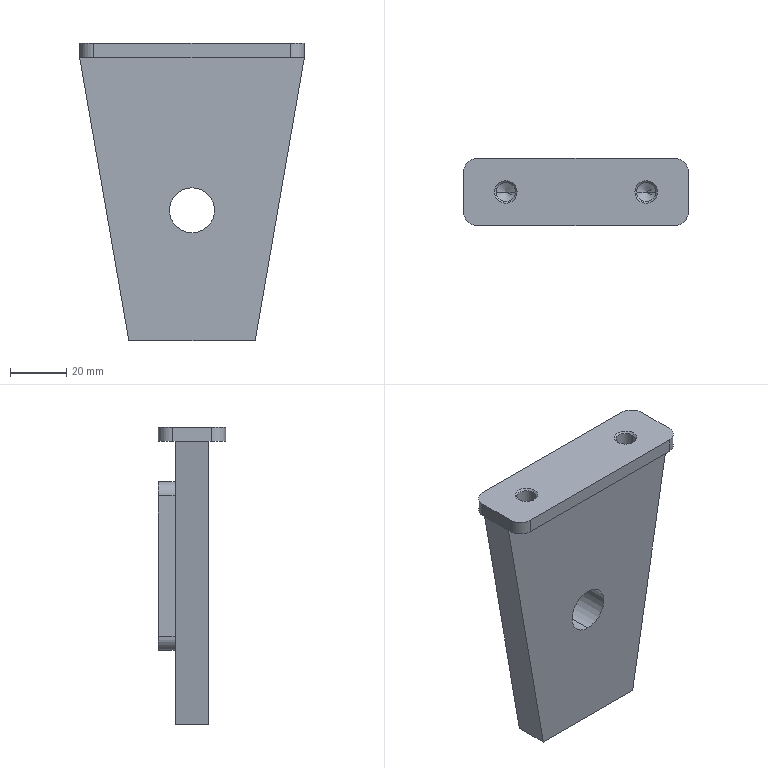Part | SolidWorks | features ICE 3, 3DProfileFeature 2, HoleWzd 2, Extrusion 1 | 1 solid | 51 faces | box 80 x 24 x 106 mm | volume 92527 mm3 | cylinder 18 | plane 17 | cone 16 | commonest cylinder face diameters 10 x8 5 x4 6.8 x4 16 x2
STEP:
#1=CARTESIAN_POINT('',(16.5,0.,-100.475));
#2=VERTEX_POINT('',#1);
#3=CARTESIAN_POINT('',(11.5,0.,-100.475));
#4=VERTEX_POINT('',#3);
#5=CARTESIAN_POINT('',(14.,0.,-100.475));
#6=DIRECTION('',(0.,0.,-1.));
#7=DIRECTION('',(-1.,0.,0.));
#8=AXIS2_PLACEMENT_3D('',#5,#6,#7);
#9=CIRCLE('',#8,2.5);
#10=EDGE_CURVE('',#2,#4,#9,.T.);
#11=ORIENTED_EDGE('',*,*,#10,.F.);
#12=CARTESIAN_POINT('',(17.025,0.,-101.));
#13=VERTEX_POINT('',#12);
#14=CARTESIAN_POINT('',(17.025,0.,-101.));
#15=DIRECTION('',(0.7071,0.,-0.7071));
#16=VECTOR('',#15,1000.);
#17=LINE('',#14,#16);
#18=EDGE_CURVE('',#2,#13,#17,.T.);
#19=ORIENTED_EDGE('',*,*,#18,.T.);
#20=CARTESIAN_POINT('',(10.975,0.,-101.));
#21=VERTEX_POINT('',#20);
#22=CARTESIAN_POINT('',(14.,0.,-101.));
#23=DIRECTION('',(0.,0.,-1.));
#24=DIRECTION('',(-1.,0.,0.));
#25=AXIS2_PLACEMENT_3D('',#22,#23,#24);
#26=CIRCLE('',#25,3.025);
#27=EDGE_CURVE('',#13,#21,#26,.T.);
#28=ORIENTED_EDGE('',*,*,#27,.T.);
#29=CARTESIAN_POINT('',(10.975,0.,-101.));
#30=DIRECTION('',(-0.7071,0.,-0.7071));
#31=VECTOR('',#30,1000.);
#32=LINE('',#29,#31);
#33=EDGE_CURVE('',#4,#21,#32,.T.);
#34=ORIENTED_EDGE('',*,*,#33,.F.);
#35=EDGE_LOOP('',(#11,#19,#28,#34));
#36=FACE_OUTER_BOUND('',#35,.T.);
#37=CARTESIAN_POINT('',(14.,0.,-101.));
#38=DIRECTION('',(0.,0.,-1.));
#39=DIRECTION('',(-1.,0.,0.));
#40=AXIS2_PLACEMENT_3D('',#37,#38,#39);
#41=CONICAL_SURFACE('',#40,3.025,0.7854);
#42=ADVANCED_FACE('',(#36),#41,.F.);
#43=CARTESIAN_POINT('',(16.5,0.,-91.));
#44=VERTEX_POINT('',#43);
#45=CARTESIAN_POINT('',(11.5,0.,-91.));
#46=VERTEX_POINT('',#45);
#47=CARTESIAN_POINT('',(14.,0.,-91.));
#48=DIRECTION('',(0.,0.,-1.));
#49=DIRECTION('',(-1.,0.,0.));
#50=AXIS2_PLACEMENT_3D('',#47,#48,#49);
#51=CIRCLE('',#50,2.5);
#52=EDGE_CURVE('',#44,#46,#51,.T.);
#53=ORIENTED_EDGE('',*,*,#52,.F.);
#54=CARTESIAN_POINT('',(16.5,0.,-101.));
#55=DIRECTION('',(0.,0.,-1.));
#56=VECTOR('',#55,1000.);
#57=LINE('',#54,#56);
#58=EDGE_CURVE('',#44,#2,#57,.T.);
#59=ORIENTED_EDGE('',*,*,#58,.T.);
#60=ORIENTED_EDGE('',*,*,#10,.T.);
#61=CARTESIAN_POINT('',(11.5,0.,-101.));
#62=DIRECTION('',(0.,0.,-1.));
#63=VECTOR('',#62,1000.);
#64=LINE('',#61,#63);
#65=EDGE_CURVE('',#46,#4,#64,.T.);
#66=ORIENTED_EDGE('',*,*,#65,.F.);
#67=EDGE_LOOP('',(#53,#59,#60,#66));
#68=FACE_OUTER_BOUND('',#67,.T.);
#69=CARTESIAN_POINT('',(14.,0.,-101.));
#70=DIRECTION('',(0.,0.,-1.));
#71=DIRECTION('',(-1.,0.,0.));
#72=AXIS2_PLACEMENT_3D('',#69,#70,#71);
#73=CYLINDRICAL_SURFACE('',#72,2.5);
#74=ADVANCED_FACE('',(#68),#73,.F.);
#75=CARTESIAN_POINT('',(14.,0.,-89.498));
#76=VERTEX_POINT('',#75);
#77=CARTESIAN_POINT('',(11.5,0.,-91.));
#78=DIRECTION('',(-0.8572,0.,-0.515));
#79=VECTOR('',#78,1000.);
#80=LINE('',#77,#79);
#81=EDGE_CURVE('',#76,#46,#80,.T.);
#82=ORIENTED_EDGE('',*,*,#81,.F.);
#83=CARTESIAN_POINT('',(16.5,0.,-91.));
#84=DIRECTION('',(0.8572,0.,-0.515));
#85=VECTOR('',#84,1000.);
#86=LINE('',#83,#85);
#87=EDGE_CURVE('',#76,#44,#86,.T.);
#88=ORIENTED_EDGE('',*,*,#87,.T.);
#89=ORIENTED_EDGE('',*,*,#52,.T.);
#90=EDGE_LOOP('',(#82,#88,#89));
#91=FACE_OUTER_BOUND('',#90,.T.);
#92=CARTESIAN_POINT('',(14.,0.,-91.));
#93=DIRECTION('',(0.,0.,-1.));
#94=DIRECTION('',(-1.,0.,0.));
#95=AXIS2_PLACEMENT_3D('',#92,#93,#94);
#96=CONICAL_SURFACE('',#95,2.5,1.03);
#97=ADVANCED_FACE('',(#91),#96,.F.);
#98=CARTESIAN_POINT('',(-11.5,0.,-100.475));
#99=VERTEX_POINT('',#98);
#100=CARTESIAN_POINT('',(-16.5,0.,-100.475));
#101=VERTEX_POINT('',#100);
#102=CARTESIAN_POINT('',(-14.,0.,-100.475));
#103=DIRECTION('',(0.,0.,-1.));
#104=DIRECTION('',(-1.,0.,0.));
#105=AXIS2_PLACEMENT_3D('',#102,#103,#104);
#106=CIRCLE('',#105,2.5);
#107=EDGE_CURVE('',#99,#101,#106,.T.);
#108=ORIENTED_EDGE('',*,*,#107,.F.);
#109=CARTESIAN_POINT('',(-10.975,0.,-101.));
#110=VERTEX_POINT('',#109);
#111=CARTESIAN_POINT('',(-10.975,0.,-101.));
#112=DIRECTION('',(0.7071,0.,-0.7071));
#113=VECTOR('',#112,1000.);
#114=LINE('',#111,#113);
#115=EDGE_CURVE('',#99,#110,#114,.T.);
#116=ORIENTED_EDGE('',*,*,#115,.T.);
#117=CARTESIAN_POINT('',(-17.025,0.,-101.));
#118=VERTEX_POINT('',#117);
#119=CARTESIAN_POINT('',(-14.,0.,-101.));
#120=DIRECTION('',(0.,0.,-1.));
#121=DIRECTION('',(-1.,0.,0.));
#122=AXIS2_PLACEMENT_3D('',#119,#120,#121);
#123=CIRCLE('',#122,3.025);
#124=EDGE_CURVE('',#110,#118,#123,.T.);
#125=ORIENTED_EDGE('',*,*,#124,.T.);
#126=CARTESIAN_POINT('',(-17.025,0.,-101.));
#127=DIRECTION('',(-0.7071,0.,-0.7071));
#128=VECTOR('',#127,1000.);
#129=LINE('',#126,#128);
#130=EDGE_CURVE('',#101,#118,#129,.T.);
#131=ORIENTED_EDGE('',*,*,#130,.F.);
#132=EDGE_LOOP('',(#108,#116,#125,#131));
#133=FACE_OUTER_BOUND('',#132,.T.);
#134=CARTESIAN_POINT('',(-14.,0.,-101.));
#135=DIRECTION('',(0.,0.,-1.));
#136=DIRECTION('',(-1.,0.,0.));
#137=AXIS2_PLACEMENT_3D('',#134,#135,#136);
#138=CONICAL_SURFACE('',#137,3.025,0.7854);
#139=ADVANCED_FACE('',(#133),#138,.F.);
#140=CARTESIAN_POINT('',(-11.5,0.,-91.));
#141=VERTEX_POINT('',#140);
#142=CARTESIAN_POINT('',(-16.5,0.,-91.));
#143=VERTEX_POINT('',#142);
#144=CARTESIAN_POINT('',(-14.,0.,-91.));
#145=DIRECTION('',(0.,0.,-1.));
#146=DIRECTION('',(-1.,0.,0.));
#147=AXIS2_PLACEMENT_3D('',#144,#145,#146);
#148=CIRCLE('',#147,2.5);
#149=EDGE_CURVE('',#141,#143,#148,.T.);
#150=ORIENTED_EDGE('',*,*,#149,.F.);
#151=CARTESIAN_POINT('',(-11.5,0.,-101.));
#152=DIRECTION('',(0.,0.,-1.));
#153=VECTOR('',#152,1000.);
#154=LINE('',#151,#153);
#155=EDGE_CURVE('',#141,#99,#154,.T.);
#156=ORIENTED_EDGE('',*,*,#155,.T.);
#157=ORIENTED_EDGE('',*,*,#107,.T.);
#158=CARTESIAN_POINT('',(-16.5,0.,-101.));
#159=DIRECTION('',(0.,0.,-1.));
#160=VECTOR('',#159,1000.);
#161=LINE('',#158,#160);
#162=EDGE_CURVE('',#143,#101,#161,.T.);
#163=ORIENTED_EDGE('',*,*,#162,.F.);
#164=EDGE_LOOP('',(#150,#156,#157,#163));
#165=FACE_OUTER_BOUND('',#164,.T.);
#166=CARTESIAN_POINT('',(-14.,0.,-101.));
#167=DIRECTION('',(0.,0.,-1.));
#168=DIRECTION('',(-1.,0.,0.));
#169=AXIS2_PLACEMENT_3D('',#166,#167,#168);
#170=CYLINDRICAL_SURFACE('',#169,2.5);
#171=ADVANCED_FACE('',(#165),#170,.F.);
#172=CARTESIAN_POINT('',(-14.,0.,-89.498));
#173=VERTEX_POINT('',#172);
#174=CARTESIAN_POINT('',(-16.5,0.,-91.));
#175=DIRECTION('',(-0.8572,0.,-0.515));
#176=VECTOR('',#175,1000.);
#177=LINE('',#174,#176);
#178=EDGE_CURVE('',#173,#143,#177,.T.);
#179=ORIENTED_EDGE('',*,*,#178,.F.);
#180=CARTESIAN_POINT('',(-11.5,0.,-91.));
#181=DIRECTION('',(0.8572,0.,-0.515));
#182=VECTOR('',#181,1000.);
#183=LINE('',#180,#182);
#184=EDGE_CURVE('',#173,#141,#183,.T.);
#185=ORIENTED_EDGE('',*,*,#184,.T.);
#186=ORIENTED_EDGE('',*,*,#149,.T.);
#187=EDGE_LOOP('',(#179,#185,#186));
#188=FACE_OUTER_BOUND('',#187,.T.);
#189=CARTESIAN_POINT('',(-14.,0.,-91.));
#190=DIRECTION('',(0.,0.,-1.));
#191=DIRECTION('',(-1.,0.,0.));
#192=AXIS2_PLACEMENT_3D('',#189,#190,#191);
#193=CONICAL_SURFACE('',#192,2.5,1.03);
#194=ADVANCED_FACE('',(#188),#193,.F.);
#195=CARTESIAN_POINT('',(21.6,0.,4.375));
#196=VERTEX_POINT('',#195);
#197=CARTESIAN_POINT('',(28.4,0.,4.375));
#198=VERTEX_POINT('',#197);
#199=CARTESIAN_POINT('',(25.,0.,4.375));
#200=DIRECTION('',(0.,0.,1.));
#201=DIRECTION('',(1.,0.,0.));
#202=AXIS2_PLACEMENT_3D('',#199,#200,#201);
#203=CIRCLE('',#202,3.4);
#204=EDGE_CURVE('',#196,#198,#203,.T.);
#205=ORIENTED_EDGE('',*,*,#204,.F.);
#206=CARTESIAN_POINT('',(20.975,0.,5.));
#207=VERTEX_POINT('',#206);
#208=CARTESIAN_POINT('',(20.975,0.,5.));
#209=DIRECTION('',(-0.7071,0.,0.7071));
#210=VECTOR('',#209,1000.);
#211=LINE('',#208,#210);
#212=EDGE_CURVE('',#196,#207,#211,.T.);
#213=ORIENTED_EDGE('',*,*,#212,.T.);
#214=CARTESIAN_POINT('',(29.025,0.,5.));
#215=VERTEX_POINT('',#214);
#216=CARTESIAN_POINT('',(25.,0.,5.));
#217=DIRECTION('',(0.,0.,1.));
#218=DIRECTION('',(1.,0.,0.));
#219=AXIS2_PLACEMENT_3D('',#216,#217,#218);
#220=CIRCLE('',#219,4.025);
#221=EDGE_CURVE('',#207,#215,#220,.T.);
#222=ORIENTED_EDGE('',*,*,#221,.T.);
#223=CARTESIAN_POINT('',(29.025,0.,5.));
#224=DIRECTION('',(0.7071,0.,0.7071));
#225=VECTOR('',#224,1000.);
#226=LINE('',#223,#225);
#227=EDGE_CURVE('',#198,#215,#226,.T.);
#228=ORIENTED_EDGE('',*,*,#227,.F.);
#229=EDGE_LOOP('',(#205,#213,#222,#228));
#230=FACE_OUTER_BOUND('',#229,.T.);
#231=CARTESIAN_POINT('',(25.,0.,5.));
#232=DIRECTION('',(0.,0.,1.));
#233=DIRECTION('',(1.,0.,0.));
#234=AXIS2_PLACEMENT_3D('',#231,#232,#233);
#235=CONICAL_SURFACE('',#234,4.025,0.7854);
#236=ADVANCED_FACE('',(#230),#235,.F.);
#237=CARTESIAN_POINT('',(21.6,0.,-15.));
#238=VERTEX_POINT('',#237);
#239=CARTESIAN_POINT('',(28.4,0.,-15.));
#240=VERTEX_POINT('',#239);
#241=CARTESIAN_POINT('',(25.,0.,-15.));
#242=DIRECTION('',(0.,0.,1.));
#243=DIRECTION('',(1.,0.,0.));
#244=AXIS2_PLACEMENT_3D('',#241,#242,#243);
#245=CIRCLE('',#244,3.4);
#246=EDGE_CURVE('',#238,#240,#245,.T.);
#247=ORIENTED_EDGE('',*,*,#246,.F.);
#248=CARTESIAN_POINT('',(21.6,0.,5.));
#249=DIRECTION('',(0.,0.,1.));
#250=VECTOR('',#249,1000.);
#251=LINE('',#248,#250);
#252=EDGE_CURVE('',#238,#196,#251,.T.);
#253=ORIENTED_EDGE('',*,*,#252,.T.);
#254=ORIENTED_EDGE('',*,*,#204,.T.);
#255=CARTESIAN_POINT('',(28.4,0.,5.));
#256=DIRECTION('',(0.,0.,1.));
#257=VECTOR('',#256,1000.);
#258=LINE('',#255,#257);
#259=EDGE_CURVE('',#240,#198,#258,.T.);
#260=ORIENTED_EDGE('',*,*,#259,.F.);
#261=EDGE_LOOP('',(#247,#253,#254,#260));
#262=FACE_OUTER_BOUND('',#261,.T.);
#263=CARTESIAN_POINT('',(25.,0.,5.));
#264=DIRECTION('',(0.,0.,1.));
#265=DIRECTION('',(1.,0.,0.));
#266=AXIS2_PLACEMENT_3D('',#263,#264,#265);
#267=CYLINDRICAL_SURFACE('',#266,3.4);
#268=ADVANCED_FACE('',(#262),#267,.F.);
#269=CARTESIAN_POINT('',(25.,0.,-17.043));
#270=VERTEX_POINT('',#269);
#271=CARTESIAN_POINT('',(28.4,0.,-15.));
#272=DIRECTION('',(0.8572,0.,0.515));
#273=VECTOR('',#272,1000.);
#274=LINE('',#271,#273);
#275=EDGE_CURVE('',#270,#240,#274,.T.);
#276=ORIENTED_EDGE('',*,*,#275,.F.);
#277=CARTESIAN_POINT('',(21.6,0.,-15.));
#278=DIRECTION('',(-0.8572,0.,0.515));
#279=VECTOR('',#278,1000.);
#280=LINE('',#277,#279);
#281=EDGE_CURVE('',#270,#238,#280,.T.);
#282=ORIENTED_EDGE('',*,*,#281,.T.);
#283=ORIENTED_EDGE('',*,*,#246,.T.);
#284=EDGE_LOOP('',(#276,#282,#283));
#285=FACE_OUTER_BOUND('',#284,.T.);
#286=CARTESIAN_POINT('',(25.,0.,-15.));
#287=DIRECTION('',(0.,0.,1.));
#288=DIRECTION('',(1.,0.,0.));
#289=AXIS2_PLACEMENT_3D('',#286,#287,#288);
#290=CONICAL_SURFACE('',#289,3.4,1.03);
#291=ADVANCED_FACE('',(#285),#290,.F.);
#292=CARTESIAN_POINT('',(-28.4,0.,4.375));
#293=VERTEX_POINT('',#292);
#294=CARTESIAN_POINT('',(-21.6,0.,4.375));
#295=VERTEX_POINT('',#294);
#296=CARTESIAN_POINT('',(-25.,0.,4.375));
#297=DIRECTION('',(0.,0.,1.));
#298=DIRECTION('',(1.,0.,0.));
#299=AXIS2_PLACEMENT_3D('',#296,#297,#298);
#300=CIRCLE('',#299,3.4);
#301=EDGE_CURVE('',#293,#295,#300,.T.);
#302=ORIENTED_EDGE('',*,*,#301,.F.);
#303=CARTESIAN_POINT('',(-29.025,0.,5.));
#304=VERTEX_POINT('',#303);
#305=CARTESIAN_POINT('',(-29.025,0.,5.));
#306=DIRECTION('',(-0.7071,0.,0.7071));
#307=VECTOR('',#306,1000.);
#308=LINE('',#305,#307);
#309=EDGE_CURVE('',#293,#304,#308,.T.);
#310=ORIENTED_EDGE('',*,*,#309,.T.);
#311=CARTESIAN_POINT('',(-20.975,0.,5.));
#312=VERTEX_POINT('',#311);
#313=CARTESIAN_POINT('',(-25.,0.,5.));
#314=DIRECTION('',(0.,0.,1.));
#315=DIRECTION('',(1.,0.,0.));
#316=AXIS2_PLACEMENT_3D('',#313,#314,#315);
#317=CIRCLE('',#316,4.025);
#318=EDGE_CURVE('',#304,#312,#317,.T.);
#319=ORIENTED_EDGE('',*,*,#318,.T.);
#320=CARTESIAN_POINT('',(-20.975,0.,5.));
#321=DIRECTION('',(0.7071,0.,0.7071));
#322=VECTOR('',#321,1000.);
#323=LINE('',#320,#322);
#324=EDGE_CURVE('',#295,#312,#323,.T.);
#325=ORIENTED_EDGE('',*,*,#324,.F.);
#326=EDGE_LOOP('',(#302,#310,#319,#325));
#327=FACE_OUTER_BOUND('',#326,.T.);
#328=CARTESIAN_POINT('',(-25.,0.,5.));
#329=DIRECTION('',(0.,0.,1.));
#330=DIRECTION('',(1.,0.,0.));
#331=AXIS2_PLACEMENT_3D('',#328,#329,#330);
#332=CONICAL_SURFACE('',#331,4.025,0.7854);
#333=ADVANCED_FACE('',(#327),#332,.F.);
#334=CARTESIAN_POINT('',(-28.4,0.,-15.));
#335=VERTEX_POINT('',#334);
#336=CARTESIAN_POINT('',(-21.6,0.,-15.));
#337=VERTEX_POINT('',#336);
#338=CARTESIAN_POINT('',(-25.,0.,-15.));
#339=DIRECTION('',(0.,0.,1.));
#340=DIRECTION('',(1.,0.,0.));
#341=AXIS2_PLACEMENT_3D('',#338,#339,#340);
#342=CIRCLE('',#341,3.4);
#343=EDGE_CURVE('',#335,#337,#342,.T.);
#344=ORIENTED_EDGE('',*,*,#343,.F.);
#345=CARTESIAN_POINT('',(-28.4,0.,5.));
#346=DIRECTION('',(0.,0.,1.));
#347=VECTOR('',#346,1000.);
#348=LINE('',#345,#347);
#349=EDGE_CURVE('',#335,#293,#348,.T.);
#350=ORIENTED_EDGE('',*,*,#349,.T.);
#351=ORIENTED_EDGE('',*,*,#301,.T.);
#352=CARTESIAN_POINT('',(-21.6,0.,5.));
#353=DIRECTION('',(0.,0.,1.));
#354=VECTOR('',#353,1000.);
#355=LINE('',#352,#354);
#356=EDGE_CURVE('',#337,#295,#355,.T.);
#357=ORIENTED_EDGE('',*,*,#356,.F.);
#358=EDGE_LOOP('',(#344,#350,#351,#357));
#359=FACE_OUTER_BOUND('',#358,.T.);
#360=CARTESIAN_POINT('',(-25.,0.,5.));
#361=DIRECTION('',(0.,0.,1.));
#362=DIRECTION('',(1.,0.,0.));
#363=AXIS2_PLACEMENT_3D('',#360,#361,#362);
#364=CYLINDRICAL_SURFACE('',#363,3.4);
#365=ADVANCED_FACE('',(#359),#364,.F.);
#366=CARTESIAN_POINT('',(-25.,0.,-17.043));
#367=VERTEX_POINT('',#366);
#368=CARTESIAN_POINT('',(-21.6,0.,-15.));
#369=DIRECTION('',(0.8572,0.,0.515));
#370=VECTOR('',#369,1000.);
#371=LINE('',#368,#370);
#372=EDGE_CURVE('',#367,#337,#371,.T.);
#373=ORIENTED_EDGE('',*,*,#372,.F.);
#374=CARTESIAN_POINT('',(-28.4,0.,-15.));
#375=DIRECTION('',(-0.8572,0.,0.515));
#376=VECTOR('',#375,1000.);
#377=LINE('',#374,#376);
#378=EDGE_CURVE('',#367,#335,#377,.T.);
#379=ORIENTED_EDGE('',*,*,#378,.T.);
#380=ORIENTED_EDGE('',*,*,#343,.T.);
#381=EDGE_LOOP('',(#373,#379,#380));
#382=FACE_OUTER_BOUND('',#381,.T.);
#383=CARTESIAN_POINT('',(-25.,0.,-15.));
#384=DIRECTION('',(0.,0.,1.));
#385=DIRECTION('',(1.,0.,0.));
#386=AXIS2_PLACEMENT_3D('',#383,#384,#385);
#387=CONICAL_SURFACE('',#386,3.4,1.03);
#388=ADVANCED_FACE('',(#382),#387,.F.);
#389=CARTESIAN_POINT('',(0.,-6.,-46.5));
#390=VERTEX_POINT('',#389);
#391=CARTESIAN_POINT('',(0.,-6.,-62.5));
#392=VERTEX_POINT('',#391);
#393=CARTESIAN_POINT('',(0.,-6.,-54.5));
#394=DIRECTION('',(0.,-1.,0.));
#395=DIRECTION('',(0.,0.,-1.));
#396=AXIS2_PLACEMENT_3D('',#393,#394,#395);
#397=CIRCLE('',#396,8.);
#398=EDGE_CURVE('',#390,#392,#397,.T.);
#399=ORIENTED_EDGE('',*,*,#398,.T.);
#400=CARTESIAN_POINT('',(0.,12.,-62.5));
#401=VERTEX_POINT('',#400);
#402=CARTESIAN_POINT('',(0.,-9.,-62.5));
#403=DIRECTION('',(0.,1.,0.));
#404=VECTOR('',#403,1000.);
#405=LINE('',#402,#404);
#406=EDGE_CURVE('',#392,#401,#405,.T.);
#407=ORIENTED_EDGE('',*,*,#406,.T.);
#408=CARTESIAN_POINT('',(0.,12.,-46.5));
#409=VERTEX_POINT('',#408);
#410=CARTESIAN_POINT('',(0.,12.,-54.5));
#411=DIRECTION('',(0.,1.,0.));
#412=DIRECTION('',(0.,0.,1.));
#413=AXIS2_PLACEMENT_3D('',#410,#411,#412);
#414=CIRCLE('',#413,8.);
#415=EDGE_CURVE('',#401,#409,#414,.T.);
#416=ORIENTED_EDGE('',*,*,#415,.T.);
#417=CARTESIAN_POINT('',(0.,-9.,-46.5));
#418=DIRECTION('',(0.,1.,0.));
#419=VECTOR('',#418,1000.);
#420=LINE('',#417,#419);
#421=EDGE_CURVE('',#390,#409,#420,.T.);
#422=ORIENTED_EDGE('',*,*,#421,.F.);
#423=EDGE_LOOP('',(#399,#407,#416,#422));
#424=FACE_OUTER_BOUND('',#423,.T.);
#425=CARTESIAN_POINT('',(0.,-9.,-54.5));
#426=DIRECTION('',(0.,1.,0.));
#427=DIRECTION('',(0.,0.,1.));
#428=AXIS2_PLACEMENT_3D('',#425,#426,#427);
#429=CYLINDRICAL_SURFACE('',#428,8.);
#430=ADVANCED_FACE('',(#424),#429,.F.);
#431=CARTESIAN_POINT('',(-40.,6.,0.));
#432=VERTEX_POINT('',#431);
#433=CARTESIAN_POINT('',(40.,6.,0.));
#434=VERTEX_POINT('',#433);
#435=CARTESIAN_POINT('',(40.,6.,0.));
#436=DIRECTION('',(1.,0.,0.));
#437=VECTOR('',#436,1000.);
#438=LINE('',#435,#437);
#439=EDGE_CURVE('',#432,#434,#438,.T.);
#440=ORIENTED_EDGE('',*,*,#439,.T.);
#441=CARTESIAN_POINT('',(22.5,6.,-101.));
#442=VERTEX_POINT('',#441);
#443=CARTESIAN_POINT('',(22.5,6.,-101.));
#444=DIRECTION('',(-0.1707,0.,-0.9853));
#445=VECTOR('',#444,1000.);
#446=LINE('',#443,#445);
#447=EDGE_CURVE('',#434,#442,#446,.T.);
#448=ORIENTED_EDGE('',*,*,#447,.T.);
#449=CARTESIAN_POINT('',(-22.5,6.,-101.));
#450=VERTEX_POINT('',#449);
#451=CARTESIAN_POINT('',(-22.5,6.,-101.));
#452=DIRECTION('',(-1.,0.,0.));
#453=VECTOR('',#452,1000.);
#454=LINE('',#451,#453);
#455=EDGE_CURVE('',#442,#450,#454,.T.);
#456=ORIENTED_EDGE('',*,*,#455,.T.);
#457=CARTESIAN_POINT('',(-40.,6.,0.));
#458=DIRECTION('',(-0.1707,0.,0.9853));
#459=VECTOR('',#458,1000.);
#460=LINE('',#457,#459);
#461=EDGE_CURVE('',#450,#432,#460,.T.);
#462=ORIENTED_EDGE('',*,*,#461,.T.);
#463=EDGE_LOOP('',(#440,#448,#456,#462));
#464=FACE_OUTER_BOUND('',#463,.T.);
#465=CARTESIAN_POINT('',(-18.,6.,-19.5));
#466=VERTEX_POINT('',#465);
#467=CARTESIAN_POINT('',(-13.,6.,-14.5));
#468=VERTEX_POINT('',#467);
#469=CARTESIAN_POINT('',(-13.,6.,-19.5));
#470=DIRECTION('',(0.,1.,0.));
#471=DIRECTION('',(0.,0.,-1.));
#472=AXIS2_PLACEMENT_3D('',#469,#470,#471);
#473=CIRCLE('',#472,5.);
#474=EDGE_CURVE('',#466,#468,#473,.T.);
#475=ORIENTED_EDGE('',*,*,#474,.F.);
#476=CARTESIAN_POINT('',(-18.,6.,-69.5));
#477=VERTEX_POINT('',#476);
#478=CARTESIAN_POINT('',(-18.,6.,-19.5));
#479=DIRECTION('',(0.,0.,1.));
#480=VECTOR('',#479,1000.);
#481=LINE('',#478,#480);
#482=EDGE_CURVE('',#477,#466,#481,.T.);
#483=ORIENTED_EDGE('',*,*,#482,.F.);
#484=CARTESIAN_POINT('',(-13.,6.,-74.5));
#485=VERTEX_POINT('',#484);
#486=CARTESIAN_POINT('',(-13.,6.,-69.5));
#487=DIRECTION('',(0.,1.,0.));
#488=DIRECTION('',(0.,0.,-1.));
#489=AXIS2_PLACEMENT_3D('',#486,#487,#488);
#490=CIRCLE('',#489,5.);
#491=EDGE_CURVE('',#485,#477,#490,.T.);
#492=ORIENTED_EDGE('',*,*,#491,.F.);
#493=CARTESIAN_POINT('',(13.,6.,-74.5));
#494=VERTEX_POINT('',#493);
#495=CARTESIAN_POINT('',(-13.,6.,-74.5));
#496=DIRECTION('',(-1.,0.,0.));
#497=VECTOR('',#496,1000.);
#498=LINE('',#495,#497);
#499=EDGE_CURVE('',#494,#485,#498,.T.);
#500=ORIENTED_EDGE('',*,*,#499,.F.);
#501=CARTESIAN_POINT('',(18.,6.,-69.5));
#502=VERTEX_POINT('',#501);
#503=CARTESIAN_POINT('',(13.,6.,-69.5));
#504=DIRECTION('',(0.,1.,0.));
#505=DIRECTION('',(0.,0.,-1.));
#506=AXIS2_PLACEMENT_3D('',#503,#504,#505);
#507=CIRCLE('',#506,5.);
#508=EDGE_CURVE('',#502,#494,#507,.T.);
#509=ORIENTED_EDGE('',*,*,#508,.F.);
#510=CARTESIAN_POINT('',(18.,6.,-19.5));
#511=VERTEX_POINT('',#510);
#512=CARTESIAN_POINT('',(18.,6.,-19.5));
#513=DIRECTION('',(0.,0.,-1.));
#514=VECTOR('',#513,1000.);
#515=LINE('',#512,#514);
#516=EDGE_CURVE('',#511,#502,#515,.T.);
#517=ORIENTED_EDGE('',*,*,#516,.F.);
#518=CARTESIAN_POINT('',(13.,6.,-14.5));
#519=VERTEX_POINT('',#518);
#520=CARTESIAN_POINT('',(13.,6.,-19.5));
#521=DIRECTION('',(0.,1.,0.));
#522=DIRECTION('',(0.,0.,1.));
#523=AXIS2_PLACEMENT_3D('',#520,#521,#522);
#524=CIRCLE('',#523,5.);
#525=EDGE_CURVE('',#519,#511,#524,.T.);
#526=ORIENTED_EDGE('',*,*,#525,.F.);
#527=CARTESIAN_POINT('',(-13.,6.,-14.5));
#528=DIRECTION('',(1.,0.,0.));
#529=VECTOR('',#528,1000.);
#530=LINE('',#527,#529);
#531=EDGE_CURVE('',#468,#519,#530,.T.);
#532=ORIENTED_EDGE('',*,*,#531,.F.);
#533=EDGE_LOOP('',(#475,#483,#492,#500,#509,#517,#526,#532));
#534=FACE_BOUND('',#533,.T.);
#535=CARTESIAN_POINT('',(0.,6.,0.));
#536=DIRECTION('',(0.,-1.,0.));
#537=DIRECTION('',(0.,0.,-1.));
#538=AXIS2_PLACEMENT_3D('',#535,#536,#537);
#539=PLANE('',#538);
#540=ADVANCED_FACE('',(#464,#534),#539,.F.);
#541=CARTESIAN_POINT('',(-40.,-6.,0.));
#542=VERTEX_POINT('',#541);
#543=CARTESIAN_POINT('',(-40.,-7.,0.));
#544=VERTEX_POINT('',#543);
#545=CARTESIAN_POINT('',(-40.,-7.,0.));
#546=DIRECTION('',(0.,-1.,0.));
#547=VECTOR('',#546,1000.);
#548=LINE('',#545,#547);
#549=EDGE_CURVE('',#542,#544,#548,.T.);
#550=ORIENTED_EDGE('',*,*,#549,.F.);
#551=CARTESIAN_POINT('',(40.,-6.,0.));
#552=VERTEX_POINT('',#551);
#553=CARTESIAN_POINT('',(40.,-6.,0.));
#554=DIRECTION('',(1.,0.,0.));
#555=VECTOR('',#554,1000.);
#556=LINE('',#553,#555);
#557=EDGE_CURVE('',#542,#552,#556,.T.);
#558=ORIENTED_EDGE('',*,*,#557,.T.);
#559=CARTESIAN_POINT('',(40.,-7.,0.));
#560=VERTEX_POINT('',#559);
#561=CARTESIAN_POINT('',(40.,-7.,0.));
#562=DIRECTION('',(0.,1.,0.));
#563=VECTOR('',#562,1000.);
#564=LINE('',#561,#563);
#565=EDGE_CURVE('',#560,#552,#564,.T.);
#566=ORIENTED_EDGE('',*,*,#565,.F.);
#567=CARTESIAN_POINT('',(35.,-12.,0.));
#568=VERTEX_POINT('',#567);
#569=CARTESIAN_POINT('',(35.,-7.,0.));
#570=DIRECTION('',(0.,0.,1.));
#571=DIRECTION('',(1.,0.,0.));
#572=AXIS2_PLACEMENT_3D('',#569,#570,#571);
#573=CIRCLE('',#572,5.);
#574=EDGE_CURVE('',#568,#560,#573,.T.);
#575=ORIENTED_EDGE('',*,*,#574,.F.);
#576=CARTESIAN_POINT('',(-35.,-12.,0.));
#577=VERTEX_POINT('',#576);
#578=CARTESIAN_POINT('',(-35.,-12.,0.));
#579=DIRECTION('',(1.,0.,0.));
#580=VECTOR('',#579,1000.);
#581=LINE('',#578,#580);
#582=EDGE_CURVE('',#577,#568,#581,.T.);
#583=ORIENTED_EDGE('',*,*,#582,.F.);
#584=CARTESIAN_POINT('',(-35.,-7.,0.));
#585=DIRECTION('',(0.,0.,1.));
#586=DIRECTION('',(-1.,0.,0.));
#587=AXIS2_PLACEMENT_3D('',#584,#585,#586);
#588=CIRCLE('',#587,5.);
#589=EDGE_CURVE('',#544,#577,#588,.T.);
#590=ORIENTED_EDGE('',*,*,#589,.F.);
#591=EDGE_LOOP('',(#550,#558,#566,#575,#583,#590));
#592=FACE_OUTER_BOUND('',#591,.T.);
#593=CARTESIAN_POINT('',(35.,7.,0.));
#594=DIRECTION('',(0.,0.,-1.));
#595=DIRECTION('',(-1.,0.,0.));
#596=AXIS2_PLACEMENT_3D('',#593,#594,#595);
#597=PLANE('',#596);
#598=ADVANCED_FACE('',(#592),#597,.T.);
#599=CARTESIAN_POINT('',(40.,7.,0.));
#600=VERTEX_POINT('',#599);
#601=CARTESIAN_POINT('',(35.,12.,0.));
#602=VERTEX_POINT('',#601);
#603=CARTESIAN_POINT('',(35.,7.,0.));
#604=DIRECTION('',(0.,0.,1.));
#605=DIRECTION('',(-1.,0.,0.));
#606=AXIS2_PLACEMENT_3D('',#603,#604,#605);
#607=CIRCLE('',#606,5.);
#608=EDGE_CURVE('',#600,#602,#607,.T.);
#609=ORIENTED_EDGE('',*,*,#608,.T.);
#610=CARTESIAN_POINT('',(35.,12.,5.));
#611=VERTEX_POINT('',#610);
#612=CARTESIAN_POINT('',(35.,12.,5.));
#613=DIRECTION('',(0.,0.,-1.));
#614=VECTOR('',#613,1000.);
#615=LINE('',#612,#614);
#616=EDGE_CURVE('',#611,#602,#615,.T.);
#617=ORIENTED_EDGE('',*,*,#616,.F.);
#618=CARTESIAN_POINT('',(40.,7.,5.));
#619=VERTEX_POINT('',#618);
#620=CARTESIAN_POINT('',(35.,7.,5.));
#621=DIRECTION('',(0.,0.,1.));
#622=DIRECTION('',(-1.,0.,0.));
#623=AXIS2_PLACEMENT_3D('',#620,#621,#622);
#624=CIRCLE('',#623,5.);
#625=EDGE_CURVE('',#619,#611,#624,.T.);
#626=ORIENTED_EDGE('',*,*,#625,.F.);
#627=CARTESIAN_POINT('',(40.,7.,5.));
#628=DIRECTION('',(0.,0.,-1.));
#629=VECTOR('',#628,1000.);
#630=LINE('',#627,#629);
#631=EDGE_CURVE('',#619,#600,#630,.T.);
#632=ORIENTED_EDGE('',*,*,#631,.T.);
#633=EDGE_LOOP('',(#609,#617,#626,#632));
#634=FACE_OUTER_BOUND('',#633,.T.);
#635=CARTESIAN_POINT('',(35.,7.,5.));
#636=DIRECTION('',(0.,0.,-1.));
#637=DIRECTION('',(-1.,0.,0.));
#638=AXIS2_PLACEMENT_3D('',#635,#636,#637);
#639=CYLINDRICAL_SURFACE('',#638,5.);
#640=ADVANCED_FACE('',(#634),#639,.T.);
#641=CARTESIAN_POINT('',(-35.,12.,0.));
#642=VERTEX_POINT('',#641);
#643=CARTESIAN_POINT('',(-35.,12.,0.));
#644=DIRECTION('',(-1.,0.,0.));
#645=VECTOR('',#644,1000.);
#646=LINE('',#643,#645);
#647=EDGE_CURVE('',#602,#642,#646,.T.);
#648=ORIENTED_EDGE('',*,*,#647,.T.);
#649=CARTESIAN_POINT('',(-35.,12.,5.));
#650=VERTEX_POINT('',#649);
#651=CARTESIAN_POINT('',(-35.,12.,5.));
#652=DIRECTION('',(0.,0.,-1.));
#653=VECTOR('',#652,1000.);
#654=LINE('',#651,#653);
#655=EDGE_CURVE('',#650,#642,#654,.T.);
#656=ORIENTED_EDGE('',*,*,#655,.F.);
#657=CARTESIAN_POINT('',(-35.,12.,5.));
#658=DIRECTION('',(-1.,0.,0.));
#659=VECTOR('',#658,1000.);
#660=LINE('',#657,#659);
#661=EDGE_CURVE('',#611,#650,#660,.T.);
#662=ORIENTED_EDGE('',*,*,#661,.F.);
#663=ORIENTED_EDGE('',*,*,#616,.T.);
#664=EDGE_LOOP('',(#648,#656,#662,#663));
#665=FACE_OUTER_BOUND('',#664,.T.);
#666=CARTESIAN_POINT('',(-35.,12.,5.));
#667=DIRECTION('',(0.,-1.,0.));
#668=DIRECTION('',(0.,0.,-1.));
#669=AXIS2_PLACEMENT_3D('',#666,#667,#668);
#670=PLANE('',#669);
#671=ADVANCED_FACE('',(#665),#670,.F.);
#672=CARTESIAN_POINT('',(-40.,7.,0.));
#673=VERTEX_POINT('',#672);
#674=CARTESIAN_POINT('',(-35.,7.,0.));
#675=DIRECTION('',(0.,0.,1.));
#676=DIRECTION('',(-1.,0.,0.));
#677=AXIS2_PLACEMENT_3D('',#674,#675,#676);
#678=CIRCLE('',#677,5.);
#679=EDGE_CURVE('',#642,#673,#678,.T.);
#680=ORIENTED_EDGE('',*,*,#679,.T.);
#681=CARTESIAN_POINT('',(-40.,7.,5.));
#682=VERTEX_POINT('',#681);
#683=CARTESIAN_POINT('',(-40.,7.,5.));
#684=DIRECTION('',(0.,0.,-1.));
#685=VECTOR('',#684,1000.);
#686=LINE('',#683,#685);
#687=EDGE_CURVE('',#682,#673,#686,.T.);
#688=ORIENTED_EDGE('',*,*,#687,.F.);
#689=CARTESIAN_POINT('',(-35.,7.,5.));
#690=DIRECTION('',(0.,0.,1.));
#691=DIRECTION('',(-1.,0.,0.));
#692=AXIS2_PLACEMENT_3D('',#689,#690,#691);
#693=CIRCLE('',#692,5.);
#694=EDGE_CURVE('',#650,#682,#693,.T.);
#695=ORIENTED_EDGE('',*,*,#694,.F.);
#696=ORIENTED_EDGE('',*,*,#655,.T.);
#697=EDGE_LOOP('',(#680,#688,#695,#696));
#698=FACE_OUTER_BOUND('',#697,.T.);
#699=CARTESIAN_POINT('',(-35.,7.,5.));
#700=DIRECTION('',(0.,0.,-1.));
#701=DIRECTION('',(-1.,0.,0.));
#702=AXIS2_PLACEMENT_3D('',#699,#700,#701);
#703=CYLINDRICAL_SURFACE('',#702,5.);
#704=ADVANCED_FACE('',(#698),#703,.T.);
#705=CARTESIAN_POINT('',(-40.,-7.,0.));
#706=DIRECTION('',(0.,-1.,0.));
#707=VECTOR('',#706,1000.);
#708=LINE('',#705,#707);
#709=EDGE_CURVE('',#673,#432,#708,.T.);
#710=ORIENTED_EDGE('',*,*,#709,.T.);
#711=CARTESIAN_POINT('',(-40.,6.,0.));
#712=DIRECTION('',(0.,-1.,0.));
#713=VECTOR('',#712,1000.);
#714=LINE('',#711,#713);
#715=EDGE_CURVE('',#432,#542,#714,.T.);
#716=ORIENTED_EDGE('',*,*,#715,.T.);
#717=ORIENTED_EDGE('',*,*,#549,.T.);
#718=CARTESIAN_POINT('',(-40.,-7.,5.));
#719=VERTEX_POINT('',#718);
#720=CARTESIAN_POINT('',(-40.,-7.,5.));
#721=DIRECTION('',(0.,0.,-1.));
#722=VECTOR('',#721,1000.);
#723=LINE('',#720,#722);
#724=EDGE_CURVE('',#719,#544,#723,.T.);
#725=ORIENTED_EDGE('',*,*,#724,.F.);
#726=CARTESIAN_POINT('',(-40.,-7.,5.));
#727=DIRECTION('',(0.,-1.,0.));
#728=VECTOR('',#727,1000.);
#729=LINE('',#726,#728);
#730=EDGE_CURVE('',#682,#719,#729,.T.);
#731=ORIENTED_EDGE('',*,*,#730,.F.);
#732=ORIENTED_EDGE('',*,*,#687,.T.);
#733=EDGE_LOOP('',(#710,#716,#717,#725,#731,#732));
#734=FACE_OUTER_BOUND('',#733,.T.);
#735=CARTESIAN_POINT('',(-40.,-7.,5.));
#736=DIRECTION('',(1.,0.,0.));
#737=DIRECTION('',(0.,0.,-1.));
#738=AXIS2_PLACEMENT_3D('',#735,#736,#737);
#739=PLANE('',#738);
#740=ADVANCED_FACE('',(#734),#739,.F.);
#741=ORIENTED_EDGE('',*,*,#589,.T.);
#742=CARTESIAN_POINT('',(-35.,-12.,5.));
#743=VERTEX_POINT('',#742);
#744=CARTESIAN_POINT('',(-35.,-12.,5.));
#745=DIRECTION('',(0.,0.,-1.));
#746=VECTOR('',#745,1000.);
#747=LINE('',#744,#746);
#748=EDGE_CURVE('',#743,#577,#747,.T.);
#749=ORIENTED_EDGE('',*,*,#748,.F.);
#750=CARTESIAN_POINT('',(-35.,-7.,5.));
#751=DIRECTION('',(0.,0.,1.));
#752=DIRECTION('',(-1.,0.,0.));
#753=AXIS2_PLACEMENT_3D('',#750,#751,#752);
#754=CIRCLE('',#753,5.);
#755=EDGE_CURVE('',#719,#743,#754,.T.);
#756=ORIENTED_EDGE('',*,*,#755,.F.);
#757=ORIENTED_EDGE('',*,*,#724,.T.);
#758=EDGE_LOOP('',(#741,#749,#756,#757));
#759=FACE_OUTER_BOUND('',#758,.T.);
#760=CARTESIAN_POINT('',(-35.,-7.,5.));
#761=DIRECTION('',(0.,0.,-1.));
#762=DIRECTION('',(-1.,0.,0.));
#763=AXIS2_PLACEMENT_3D('',#760,#761,#762);
#764=CYLINDRICAL_SURFACE('',#763,5.);
#765=ADVANCED_FACE('',(#759),#764,.T.);
#766=ORIENTED_EDGE('',*,*,#582,.T.);
#767=CARTESIAN_POINT('',(35.,-12.,5.));
#768=VERTEX_POINT('',#767);
#769=CARTESIAN_POINT('',(35.,-12.,5.));
#770=DIRECTION('',(0.,0.,-1.));
#771=VECTOR('',#770,1000.);
#772=LINE('',#769,#771);
#773=EDGE_CURVE('',#768,#568,#772,.T.);
#774=ORIENTED_EDGE('',*,*,#773,.F.);
#775=CARTESIAN_POINT('',(-35.,-12.,5.));
#776=DIRECTION('',(1.,0.,0.));
#777=VECTOR('',#776,1000.);
#778=LINE('',#775,#777);
#779=EDGE_CURVE('',#743,#768,#778,.T.);
#780=ORIENTED_EDGE('',*,*,#779,.F.);
#781=ORIENTED_EDGE('',*,*,#748,.T.);
#782=EDGE_LOOP('',(#766,#774,#780,#781));
#783=FACE_OUTER_BOUND('',#782,.T.);
#784=CARTESIAN_POINT('',(-35.,-12.,5.));
#785=DIRECTION('',(0.,1.,0.));
#786=DIRECTION('',(0.,0.,1.));
#787=AXIS2_PLACEMENT_3D('',#784,#785,#786);
#788=PLANE('',#787);
#789=ADVANCED_FACE('',(#783),#788,.F.);
#790=ORIENTED_EDGE('',*,*,#574,.T.);
#791=CARTESIAN_POINT('',(40.,-7.,5.));
#792=VERTEX_POINT('',#791);
#793=CARTESIAN_POINT('',(40.,-7.,5.));
#794=DIRECTION('',(0.,0.,-1.));
#795=VECTOR('',#794,1000.);
#796=LINE('',#793,#795);
#797=EDGE_CURVE('',#792,#560,#796,.T.);
#798=ORIENTED_EDGE('',*,*,#797,.F.);
#799=CARTESIAN_POINT('',(35.,-7.,5.));
#800=DIRECTION('',(0.,0.,1.));
#801=DIRECTION('',(1.,0.,0.));
#802=AXIS2_PLACEMENT_3D('',#799,#800,#801);
#803=CIRCLE('',#802,5.);
#804=EDGE_CURVE('',#768,#792,#803,.T.);
#805=ORIENTED_EDGE('',*,*,#804,.F.);
#806=ORIENTED_EDGE('',*,*,#773,.T.);
#807=EDGE_LOOP('',(#790,#798,#805,#806));
#808=FACE_OUTER_BOUND('',#807,.T.);
#809=CARTESIAN_POINT('',(35.,-7.,5.));
#810=DIRECTION('',(0.,0.,-1.));
#811=DIRECTION('',(-1.,0.,0.));
#812=AXIS2_PLACEMENT_3D('',#809,#810,#811);
#813=CYLINDRICAL_SURFACE('',#812,5.);
#814=ADVANCED_FACE('',(#808),#813,.T.);
#815=ORIENTED_EDGE('',*,*,#565,.T.);
#816=CARTESIAN_POINT('',(40.,6.,0.));
#817=DIRECTION('',(0.,-1.,0.));
#818=VECTOR('',#817,1000.);
#819=LINE('',#816,#818);
#820=EDGE_CURVE('',#434,#552,#819,.T.);
#821=ORIENTED_EDGE('',*,*,#820,.F.);
#822=CARTESIAN_POINT('',(40.,-7.,0.));
#823=DIRECTION('',(0.,1.,0.));
#824=VECTOR('',#823,1000.);
#825=LINE('',#822,#824);
#826=EDGE_CURVE('',#434,#600,#825,.T.);
#827=ORIENTED_EDGE('',*,*,#826,.T.);
#828=ORIENTED_EDGE('',*,*,#631,.F.);
#829=CARTESIAN_POINT('',(40.,-7.,5.));
#830=DIRECTION('',(0.,1.,0.));
#831=VECTOR('',#830,1000.);
#832=LINE('',#829,#831);
#833=EDGE_CURVE('',#792,#619,#832,.T.);
#834=ORIENTED_EDGE('',*,*,#833,.F.);
#835=ORIENTED_EDGE('',*,*,#797,.T.);
#836=EDGE_LOOP('',(#815,#821,#827,#828,#834,#835));
#837=FACE_OUTER_BOUND('',#836,.T.);
#838=CARTESIAN_POINT('',(40.,-7.,5.));
#839=DIRECTION('',(-1.,0.,0.));
#840=DIRECTION('',(0.,0.,1.));
#841=AXIS2_PLACEMENT_3D('',#838,#839,#840);
#842=PLANE('',#841);
#843=ADVANCED_FACE('',(#837),#842,.F.);
#844=CARTESIAN_POINT('',(25.,0.,5.));
#845=DIRECTION('',(0.,0.,1.));
#846=DIRECTION('',(1.,0.,0.));
#847=AXIS2_PLACEMENT_3D('',#844,#845,#846);
#848=CIRCLE('',#847,4.025);
#849=EDGE_CURVE('',#215,#207,#848,.T.);
#850=ORIENTED_EDGE('',*,*,#849,.F.);
#851=ORIENTED_EDGE('',*,*,#221,.F.);
#852=EDGE_LOOP('',(#850,#851));
#853=FACE_BOUND('',#852,.T.);
#854=CARTESIAN_POINT('',(-25.,0.,5.));
#855=DIRECTION('',(0.,0.,1.));
#856=DIRECTION('',(1.,0.,0.));
#857=AXIS2_PLACEMENT_3D('',#854,#855,#856);
#858=CIRCLE('',#857,4.025);
#859=EDGE_CURVE('',#312,#304,#858,.T.);
#860=ORIENTED_EDGE('',*,*,#859,.F.);
#861=ORIENTED_EDGE('',*,*,#318,.F.);
#862=EDGE_LOOP('',(#860,#861));
#863=FACE_BOUND('',#862,.T.);
#864=ORIENTED_EDGE('',*,*,#625,.T.);
#865=ORIENTED_EDGE('',*,*,#661,.T.);
#866=ORIENTED_EDGE('',*,*,#694,.T.);
#867=ORIENTED_EDGE('',*,*,#730,.T.);
#868=ORIENTED_EDGE('',*,*,#755,.T.);
#869=ORIENTED_EDGE('',*,*,#779,.T.);
#870=ORIENTED_EDGE('',*,*,#804,.T.);
#871=ORIENTED_EDGE('',*,*,#833,.T.);
#872=EDGE_LOOP('',(#864,#865,#866,#867,#868,#869,#870,#871));
#873=FACE_OUTER_BOUND('',#872,.T.);
#874=CARTESIAN_POINT('',(35.,7.,5.));
#875=DIRECTION('',(0.,0.,-1.));
#876=DIRECTION('',(-1.,0.,0.));
#877=AXIS2_PLACEMENT_3D('',#874,#875,#876);
#878=PLANE('',#877);
#879=ADVANCED_FACE('',(#853,#863,#873),#878,.F.);
#880=ORIENTED_EDGE('',*,*,#439,.F.);
#881=ORIENTED_EDGE('',*,*,#709,.F.);
#882=ORIENTED_EDGE('',*,*,#679,.F.);
#883=ORIENTED_EDGE('',*,*,#647,.F.);
#884=ORIENTED_EDGE('',*,*,#608,.F.);
#885=ORIENTED_EDGE('',*,*,#826,.F.);
#886=EDGE_LOOP('',(#880,#881,#882,#883,#884,#885));
#887=FACE_OUTER_BOUND('',#886,.T.);
#888=CARTESIAN_POINT('',(35.,7.,0.));
#889=DIRECTION('',(0.,0.,-1.));
#890=DIRECTION('',(-1.,0.,0.));
#891=AXIS2_PLACEMENT_3D('',#888,#889,#890);
#892=PLANE('',#891);
#893=ADVANCED_FACE('',(#887),#892,.T.);
#894=CARTESIAN_POINT('',(22.5,-6.,-101.));
#895=VERTEX_POINT('',#894);
#896=CARTESIAN_POINT('',(22.5,-6.,-101.));
#897=DIRECTION('',(-0.1707,0.,-0.9853));
#898=VECTOR('',#897,1000.);
#899=LINE('',#896,#898);
#900=EDGE_CURVE('',#552,#895,#899,.T.);
#901=ORIENTED_EDGE('',*,*,#900,.T.);
#902=CARTESIAN_POINT('',(22.5,6.,-101.));
#903=DIRECTION('',(0.,-1.,0.));
#904=VECTOR('',#903,1000.);
#905=LINE('',#902,#904);
#906=EDGE_CURVE('',#442,#895,#905,.T.);
#907=ORIENTED_EDGE('',*,*,#906,.F.);
#908=ORIENTED_EDGE('',*,*,#447,.F.);
#909=ORIENTED_EDGE('',*,*,#820,.T.);
#910=EDGE_LOOP('',(#901,#907,#908,#909));
#911=FACE_OUTER_BOUND('',#910,.T.);
#912=CARTESIAN_POINT('',(22.5,6.,-101.));
#913=DIRECTION('',(-0.9853,0.,0.1707));
#914=DIRECTION('',(0.1707,0.,0.9853));
#915=AXIS2_PLACEMENT_3D('',#912,#913,#914);
#916=PLANE('',#915);
#917=ADVANCED_FACE('',(#911),#916,.F.);
#918=CARTESIAN_POINT('',(14.,0.,-101.));
#919=DIRECTION('',(0.,0.,-1.));
#920=DIRECTION('',(-1.,0.,0.));
#921=AXIS2_PLACEMENT_3D('',#918,#919,#920);
#922=CIRCLE('',#921,3.025);
#923=EDGE_CURVE('',#21,#13,#922,.T.);
#924=ORIENTED_EDGE('',*,*,#923,.F.);
#925=ORIENTED_EDGE('',*,*,#27,.F.);
#926=EDGE_LOOP('',(#924,#925));
#927=FACE_BOUND('',#926,.T.);
#928=CARTESIAN_POINT('',(-14.,0.,-101.));
#929=DIRECTION('',(0.,0.,-1.));
#930=DIRECTION('',(-1.,0.,0.));
#931=AXIS2_PLACEMENT_3D('',#928,#929,#930);
#932=CIRCLE('',#931,3.025);
#933=EDGE_CURVE('',#118,#110,#932,.T.);
#934=ORIENTED_EDGE('',*,*,#933,.F.);
#935=ORIENTED_EDGE('',*,*,#124,.F.);
#936=EDGE_LOOP('',(#934,#935));
#937=FACE_BOUND('',#936,.T.);
#938=CARTESIAN_POINT('',(-22.5,-6.,-101.));
#939=VERTEX_POINT('',#938);
#940=CARTESIAN_POINT('',(-22.5,-6.,-101.));
#941=DIRECTION('',(-1.,0.,0.));
#942=VECTOR('',#941,1000.);
#943=LINE('',#940,#942);
#944=EDGE_CURVE('',#895,#939,#943,.T.);
#945=ORIENTED_EDGE('',*,*,#944,.T.);
#946=CARTESIAN_POINT('',(-22.5,6.,-101.));
#947=DIRECTION('',(0.,-1.,0.));
#948=VECTOR('',#947,1000.);
#949=LINE('',#946,#948);
#950=EDGE_CURVE('',#450,#939,#949,.T.);
#951=ORIENTED_EDGE('',*,*,#950,.F.);
#952=ORIENTED_EDGE('',*,*,#455,.F.);
#953=ORIENTED_EDGE('',*,*,#906,.T.);
#954=EDGE_LOOP('',(#945,#951,#952,#953));
#955=FACE_OUTER_BOUND('',#954,.T.);
#956=CARTESIAN_POINT('',(-22.5,6.,-101.));
#957=DIRECTION('',(0.,0.,1.));
#958=DIRECTION('',(1.,0.,0.));
#959=AXIS2_PLACEMENT_3D('',#956,#957,#958);
#960=PLANE('',#959);
#961=ADVANCED_FACE('',(#927,#937,#955),#960,.F.);
#962=CARTESIAN_POINT('',(-40.,-6.,0.));
#963=DIRECTION('',(-0.1707,0.,0.9853));
#964=VECTOR('',#963,1000.);
#965=LINE('',#962,#964);
#966=EDGE_CURVE('',#939,#542,#965,.T.);
#967=ORIENTED_EDGE('',*,*,#966,.T.);
#968=ORIENTED_EDGE('',*,*,#715,.F.);
#969=ORIENTED_EDGE('',*,*,#461,.F.);
#970=ORIENTED_EDGE('',*,*,#950,.T.);
#971=EDGE_LOOP('',(#967,#968,#969,#970));
#972=FACE_OUTER_BOUND('',#971,.T.);
#973=CARTESIAN_POINT('',(-40.,6.,0.));
#974=DIRECTION('',(0.9853,0.,0.1707));
#975=DIRECTION('',(0.1707,0.,-0.9853));
#976=AXIS2_PLACEMENT_3D('',#973,#974,#975);
#977=PLANE('',#976);
#978=ADVANCED_FACE('',(#972),#977,.F.);
#979=ORIENTED_EDGE('',*,*,#398,.F.);
#980=CARTESIAN_POINT('',(0.,-6.,-54.5));
#981=DIRECTION('',(0.,-1.,0.));
#982=DIRECTION('',(0.,0.,-1.));
#983=AXIS2_PLACEMENT_3D('',#980,#981,#982);
#984=CIRCLE('',#983,8.);
#985=EDGE_CURVE('',#392,#390,#984,.T.);
#986=ORIENTED_EDGE('',*,*,#985,.F.);
#987=EDGE_LOOP('',(#979,#986));
#988=FACE_BOUND('',#987,.T.);
#989=ORIENTED_EDGE('',*,*,#557,.F.);
#990=ORIENTED_EDGE('',*,*,#966,.F.);
#991=ORIENTED_EDGE('',*,*,#944,.F.);
#992=ORIENTED_EDGE('',*,*,#900,.F.);
#993=EDGE_LOOP('',(#989,#990,#991,#992));
#994=FACE_OUTER_BOUND('',#993,.T.);
#995=CARTESIAN_POINT('',(0.,-6.,0.));
#996=DIRECTION('',(0.,-1.,0.));
#997=DIRECTION('',(0.,0.,-1.));
#998=AXIS2_PLACEMENT_3D('',#995,#996,#997);
#999=PLANE('',#998);
#1000=ADVANCED_FACE('',(#988,#994),#999,.T.);
#1001=ORIENTED_EDGE('',*,*,#474,.T.);
#1002=CARTESIAN_POINT('',(-13.,12.,-14.5));
#1003=VERTEX_POINT('',#1002);
#1004=CARTESIAN_POINT('',(-13.,12.,-14.5));
#1005=DIRECTION('',(0.,-1.,0.));
#1006=VECTOR('',#1005,1000.);
#1007=LINE('',#1004,#1006);
#1008=EDGE_CURVE('',#1003,#468,#1007,.T.);
#1009=ORIENTED_EDGE('',*,*,#1008,.F.);
#1010=CARTESIAN_POINT('',(-18.,12.,-19.5));
#1011=VERTEX_POINT('',#1010);
#1012=CARTESIAN_POINT('',(-13.,12.,-19.5));
#1013=DIRECTION('',(0.,1.,0.));
#1014=DIRECTION('',(0.,0.,-1.));
#1015=AXIS2_PLACEMENT_3D('',#1012,#1013,#1014);
#1016=CIRCLE('',#1015,5.);
#1017=EDGE_CURVE('',#1011,#1003,#1016,.T.);
#1018=ORIENTED_EDGE('',*,*,#1017,.F.);
#1019=CARTESIAN_POINT('',(-18.,12.,-19.5));
#1020=DIRECTION('',(0.,-1.,0.));
#1021=VECTOR('',#1020,1000.);
#1022=LINE('',#1019,#1021);
#1023=EDGE_CURVE('',#1011,#466,#1022,.T.);
#1024=ORIENTED_EDGE('',*,*,#1023,.T.);
#1025=EDGE_LOOP('',(#1001,#1009,#1018,#1024));
#1026=FACE_OUTER_BOUND('',#1025,.T.);
#1027=CARTESIAN_POINT('',(-13.,12.,-19.5));
#1028=DIRECTION('',(0.,-1.,0.));
#1029=DIRECTION('',(0.,0.,-1.));
#1030=AXIS2_PLACEMENT_3D('',#1027,#1028,#1029);
#1031=CYLINDRICAL_SURFACE('',#1030,5.);
#1032=ADVANCED_FACE('',(#1026),#1031,.T.);
#1033=ORIENTED_EDGE('',*,*,#531,.T.);
#1034=CARTESIAN_POINT('',(13.,12.,-14.5));
#1035=VERTEX_POINT('',#1034);
#1036=CARTESIAN_POINT('',(13.,12.,-14.5));
#1037=DIRECTION('',(0.,-1.,0.));
#1038=VECTOR('',#1037,1000.);
#1039=LINE('',#1036,#1038);
#1040=EDGE_CURVE('',#1035,#519,#1039,.T.);
#1041=ORIENTED_EDGE('',*,*,#1040,.F.);
#1042=CARTESIAN_POINT('',(-13.,12.,-14.5));
#1043=DIRECTION('',(1.,0.,0.));
#1044=VECTOR('',#1043,1000.);
#1045=LINE('',#1042,#1044);
#1046=EDGE_CURVE('',#1003,#1035,#1045,.T.);
#1047=ORIENTED_EDGE('',*,*,#1046,.F.);
#1048=ORIENTED_EDGE('',*,*,#1008,.T.);
#1049=EDGE_LOOP('',(#1033,#1041,#1047,#1048));
#1050=FACE_OUTER_BOUND('',#1049,.T.);
#1051=CARTESIAN_POINT('',(-13.,12.,-14.5));
#1052=DIRECTION('',(0.,0.,-1.));
#1053=DIRECTION('',(-1.,0.,0.));
#1054=AXIS2_PLACEMENT_3D('',#1051,#1052,#1053);
#1055=PLANE('',#1054);
#1056=ADVANCED_FACE('',(#1050),#1055,.F.);
#1057=ORIENTED_EDGE('',*,*,#525,.T.);
#1058=CARTESIAN_POINT('',(18.,12.,-19.5));
#1059=VERTEX_POINT('',#1058);
#1060=CARTESIAN_POINT('',(18.,12.,-19.5));
#1061=DIRECTION('',(0.,-1.,0.));
#1062=VECTOR('',#1061,1000.);
#1063=LINE('',#1060,#1062);
#1064=EDGE_CURVE('',#1059,#511,#1063,.T.);
#1065=ORIENTED_EDGE('',*,*,#1064,.F.);
#1066=CARTESIAN_POINT('',(13.,12.,-19.5));
#1067=DIRECTION('',(0.,1.,0.));
#1068=DIRECTION('',(0.,0.,1.));
#1069=AXIS2_PLACEMENT_3D('',#1066,#1067,#1068);
#1070=CIRCLE('',#1069,5.);
#1071=EDGE_CURVE('',#1035,#1059,#1070,.T.);
#1072=ORIENTED_EDGE('',*,*,#1071,.F.);
#1073=ORIENTED_EDGE('',*,*,#1040,.T.);
#1074=EDGE_LOOP('',(#1057,#1065,#1072,#1073));
#1075=FACE_OUTER_BOUND('',#1074,.T.);
#1076=CARTESIAN_POINT('',(13.,12.,-19.5));
#1077=DIRECTION('',(0.,-1.,0.));
#1078=DIRECTION('',(0.,0.,-1.));
#1079=AXIS2_PLACEMENT_3D('',#1076,#1077,#1078);
#1080=CYLINDRICAL_SURFACE('',#1079,5.);
#1081=ADVANCED_FACE('',(#1075),#1080,.T.);
#1082=ORIENTED_EDGE('',*,*,#516,.T.);
#1083=CARTESIAN_POINT('',(18.,12.,-69.5));
#1084=VERTEX_POINT('',#1083);
#1085=CARTESIAN_POINT('',(18.,12.,-69.5));
#1086=DIRECTION('',(0.,-1.,0.));
#1087=VECTOR('',#1086,1000.);
#1088=LINE('',#1085,#1087);
#1089=EDGE_CURVE('',#1084,#502,#1088,.T.);
#1090=ORIENTED_EDGE('',*,*,#1089,.F.);
#1091=CARTESIAN_POINT('',(18.,12.,-19.5));
#1092=DIRECTION('',(0.,0.,-1.));
#1093=VECTOR('',#1092,1000.);
#1094=LINE('',#1091,#1093);
#1095=EDGE_CURVE('',#1059,#1084,#1094,.T.);
#1096=ORIENTED_EDGE('',*,*,#1095,.F.);
#1097=ORIENTED_EDGE('',*,*,#1064,.T.);
#1098=EDGE_LOOP('',(#1082,#1090,#1096,#1097));
#1099=FACE_OUTER_BOUND('',#1098,.T.);
#1100=CARTESIAN_POINT('',(18.,12.,-19.5));
#1101=DIRECTION('',(-1.,0.,0.));
#1102=DIRECTION('',(0.,0.,1.));
#1103=AXIS2_PLACEMENT_3D('',#1100,#1101,#1102);
#1104=PLANE('',#1103);
#1105=ADVANCED_FACE('',(#1099),#1104,.F.);
#1106=ORIENTED_EDGE('',*,*,#508,.T.);
#1107=CARTESIAN_POINT('',(13.,12.,-74.5));
#1108=VERTEX_POINT('',#1107);
#1109=CARTESIAN_POINT('',(13.,12.,-74.5));
#1110=DIRECTION('',(0.,-1.,0.));
#1111=VECTOR('',#1110,1000.);
#1112=LINE('',#1109,#1111);
#1113=EDGE_CURVE('',#1108,#494,#1112,.T.);
#1114=ORIENTED_EDGE('',*,*,#1113,.F.);
#1115=CARTESIAN_POINT('',(13.,12.,-69.5));
#1116=DIRECTION('',(0.,1.,0.));
#1117=DIRECTION('',(0.,0.,-1.));
#1118=AXIS2_PLACEMENT_3D('',#1115,#1116,#1117);
#1119=CIRCLE('',#1118,5.);
#1120=EDGE_CURVE('',#1084,#1108,#1119,.T.);
#1121=ORIENTED_EDGE('',*,*,#1120,.F.);
#1122=ORIENTED_EDGE('',*,*,#1089,.T.);
#1123=EDGE_LOOP('',(#1106,#1114,#1121,#1122));
#1124=FACE_OUTER_BOUND('',#1123,.T.);
#1125=CARTESIAN_POINT('',(13.,12.,-69.5));
#1126=DIRECTION('',(0.,-1.,0.));
#1127=DIRECTION('',(0.,0.,-1.));
#1128=AXIS2_PLACEMENT_3D('',#1125,#1126,#1127);
#1129=CYLINDRICAL_SURFACE('',#1128,5.);
#1130=ADVANCED_FACE('',(#1124),#1129,.T.);
#1131=ORIENTED_EDGE('',*,*,#499,.T.);
#1132=CARTESIAN_POINT('',(-13.,12.,-74.5));
#1133=VERTEX_POINT('',#1132);
#1134=CARTESIAN_POINT('',(-13.,12.,-74.5));
#1135=DIRECTION('',(0.,-1.,0.));
#1136=VECTOR('',#1135,1000.);
#1137=LINE('',#1134,#1136);
#1138=EDGE_CURVE('',#1133,#485,#1137,.T.);
#1139=ORIENTED_EDGE('',*,*,#1138,.F.);
#1140=CARTESIAN_POINT('',(-13.,12.,-74.5));
#1141=DIRECTION('',(-1.,0.,0.));
#1142=VECTOR('',#1141,1000.);
#1143=LINE('',#1140,#1142);
#1144=EDGE_CURVE('',#1108,#1133,#1143,.T.);
#1145=ORIENTED_EDGE('',*,*,#1144,.F.);
#1146=ORIENTED_EDGE('',*,*,#1113,.T.);
#1147=EDGE_LOOP('',(#1131,#1139,#1145,#1146));
#1148=FACE_OUTER_BOUND('',#1147,.T.);
#1149=CARTESIAN_POINT('',(-13.,12.,-74.5));
#1150=DIRECTION('',(0.,0.,1.));
#1151=DIRECTION('',(1.,0.,0.));
#1152=AXIS2_PLACEMENT_3D('',#1149,#1150,#1151);
#1153=PLANE('',#1152);
#1154=ADVANCED_FACE('',(#1148),#1153,.F.);
#1155=ORIENTED_EDGE('',*,*,#491,.T.);
#1156=CARTESIAN_POINT('',(-18.,12.,-69.5));
#1157=VERTEX_POINT('',#1156);
#1158=CARTESIAN_POINT('',(-18.,12.,-69.5));
#1159=DIRECTION('',(0.,-1.,0.));
#1160=VECTOR('',#1159,1000.);
#1161=LINE('',#1158,#1160);
#1162=EDGE_CURVE('',#1157,#477,#1161,.T.);
#1163=ORIENTED_EDGE('',*,*,#1162,.F.);
#1164=CARTESIAN_POINT('',(-13.,12.,-69.5));
#1165=DIRECTION('',(0.,1.,0.));
#1166=DIRECTION('',(0.,0.,-1.));
#1167=AXIS2_PLACEMENT_3D('',#1164,#1165,#1166);
#1168=CIRCLE('',#1167,5.);
#1169=EDGE_CURVE('',#1133,#1157,#1168,.T.);
#1170=ORIENTED_EDGE('',*,*,#1169,.F.);
#1171=ORIENTED_EDGE('',*,*,#1138,.T.);
#1172=EDGE_LOOP('',(#1155,#1163,#1170,#1171));
#1173=FACE_OUTER_BOUND('',#1172,.T.);
#1174=CARTESIAN_POINT('',(-13.,12.,-69.5));
#1175=DIRECTION('',(0.,-1.,0.));
#1176=DIRECTION('',(0.,0.,-1.));
#1177=AXIS2_PLACEMENT_3D('',#1174,#1175,#1176);
#1178=CYLINDRICAL_SURFACE('',#1177,5.);
#1179=ADVANCED_FACE('',(#1173),#1178,.T.);
#1180=ORIENTED_EDGE('',*,*,#482,.T.);
#1181=ORIENTED_EDGE('',*,*,#1023,.F.);
#1182=CARTESIAN_POINT('',(-18.,12.,-19.5));
#1183=DIRECTION('',(0.,0.,1.));
#1184=VECTOR('',#1183,1000.);
#1185=LINE('',#1182,#1184);
#1186=EDGE_CURVE('',#1157,#1011,#1185,.T.);
#1187=ORIENTED_EDGE('',*,*,#1186,.F.);
#1188=ORIENTED_EDGE('',*,*,#1162,.T.);
#1189=EDGE_LOOP('',(#1180,#1181,#1187,#1188));
#1190=FACE_OUTER_BOUND('',#1189,.T.);
#1191=CARTESIAN_POINT('',(-18.,12.,-19.5));
#1192=DIRECTION('',(1.,0.,0.));
#1193=DIRECTION('',(0.,0.,-1.));
#1194=AXIS2_PLACEMENT_3D('',#1191,#1192,#1193);
#1195=PLANE('',#1194);
#1196=ADVANCED_FACE('',(#1190),#1195,.F.);
#1197=CARTESIAN_POINT('',(0.,12.,-54.5));
#1198=DIRECTION('',(0.,1.,0.));
#1199=DIRECTION('',(0.,0.,1.));
#1200=AXIS2_PLACEMENT_3D('',#1197,#1198,#1199);
#1201=CIRCLE('',#1200,8.);
#1202=EDGE_CURVE('',#409,#401,#1201,.T.);
#1203=ORIENTED_EDGE('',*,*,#1202,.F.);
#1204=ORIENTED_EDGE('',*,*,#415,.F.);
#1205=EDGE_LOOP('',(#1203,#1204));
#1206=FACE_BOUND('',#1205,.T.);
#1207=ORIENTED_EDGE('',*,*,#1017,.T.);
#1208=ORIENTED_EDGE('',*,*,#1046,.T.);
#1209=ORIENTED_EDGE('',*,*,#1071,.T.);
#1210=ORIENTED_EDGE('',*,*,#1095,.T.);
#1211=ORIENTED_EDGE('',*,*,#1120,.T.);
#1212=ORIENTED_EDGE('',*,*,#1144,.T.);
#1213=ORIENTED_EDGE('',*,*,#1169,.T.);
#1214=ORIENTED_EDGE('',*,*,#1186,.T.);
#1215=EDGE_LOOP('',(#1207,#1208,#1209,#1210,#1211,#1212,#1213,#1214));
#1216=FACE_OUTER_BOUND('',#1215,.T.);
#1217=CARTESIAN_POINT('',(-13.,12.,-19.5));
#1218=DIRECTION('',(0.,-1.,0.));
#1219=DIRECTION('',(0.,0.,-1.));
#1220=AXIS2_PLACEMENT_3D('',#1217,#1218,#1219);
#1221=PLANE('',#1220);
#1222=ADVANCED_FACE('',(#1206,#1216),#1221,.F.);
#1223=ORIENTED_EDGE('',*,*,#406,.F.);
#1224=ORIENTED_EDGE('',*,*,#985,.T.);
#1225=ORIENTED_EDGE('',*,*,#421,.T.);
#1226=ORIENTED_EDGE('',*,*,#1202,.T.);
#1227=EDGE_LOOP('',(#1223,#1224,#1225,#1226));
#1228=FACE_OUTER_BOUND('',#1227,.T.);
#1229=CARTESIAN_POINT('',(0.,-9.,-54.5));
#1230=DIRECTION('',(0.,1.,0.));
#1231=DIRECTION('',(0.,0.,1.));
#1232=AXIS2_PLACEMENT_3D('',#1229,#1230,#1231);
#1233=CYLINDRICAL_SURFACE('',#1232,8.);
#1234=ADVANCED_FACE('',(#1228),#1233,.F.);
#1235=ORIENTED_EDGE('',*,*,#378,.F.);
#1236=ORIENTED_EDGE('',*,*,#372,.T.);
#1237=CARTESIAN_POINT('',(-25.,0.,-15.));
#1238=DIRECTION('',(0.,0.,1.));
#1239=DIRECTION('',(1.,0.,0.));
#1240=AXIS2_PLACEMENT_3D('',#1237,#1238,#1239);
#1241=CIRCLE('',#1240,3.4);
#1242=EDGE_CURVE('',#337,#335,#1241,.T.);
#1243=ORIENTED_EDGE('',*,*,#1242,.T.);
#1244=EDGE_LOOP('',(#1235,#1236,#1243));
#1245=FACE_OUTER_BOUND('',#1244,.T.);
#1246=CARTESIAN_POINT('',(-25.,0.,-15.));
#1247=DIRECTION('',(0.,0.,1.));
#1248=DIRECTION('',(1.,0.,0.));
#1249=AXIS2_PLACEMENT_3D('',#1246,#1247,#1248);
#1250=CONICAL_SURFACE('',#1249,3.4,1.03);
#1251=ADVANCED_FACE('',(#1245),#1250,.F.);
#1252=ORIENTED_EDGE('',*,*,#349,.F.);
#1253=ORIENTED_EDGE('',*,*,#1242,.F.);
#1254=ORIENTED_EDGE('',*,*,#356,.T.);
#1255=CARTESIAN_POINT('',(-25.,0.,4.375));
#1256=DIRECTION('',(0.,0.,1.));
#1257=DIRECTION('',(1.,0.,0.));
#1258=AXIS2_PLACEMENT_3D('',#1255,#1256,#1257);
#1259=CIRCLE('',#1258,3.4);
#1260=EDGE_CURVE('',#295,#293,#1259,.T.);
#1261=ORIENTED_EDGE('',*,*,#1260,.T.);
#1262=EDGE_LOOP('',(#1252,#1253,#1254,#1261));
#1263=FACE_OUTER_BOUND('',#1262,.T.);
#1264=CARTESIAN_POINT('',(-25.,0.,5.));
#1265=DIRECTION('',(0.,0.,1.));
#1266=DIRECTION('',(1.,0.,0.));
#1267=AXIS2_PLACEMENT_3D('',#1264,#1265,#1266);
#1268=CYLINDRICAL_SURFACE('',#1267,3.4);
#1269=ADVANCED_FACE('',(#1263),#1268,.F.);
#1270=ORIENTED_EDGE('',*,*,#309,.F.);
#1271=ORIENTED_EDGE('',*,*,#1260,.F.);
#1272=ORIENTED_EDGE('',*,*,#324,.T.);
#1273=ORIENTED_EDGE('',*,*,#859,.T.);
#1274=EDGE_LOOP('',(#1270,#1271,#1272,#1273));
#1275=FACE_OUTER_BOUND('',#1274,.T.);
#1276=CARTESIAN_POINT('',(-25.,0.,5.));
#1277=DIRECTION('',(0.,0.,1.));
#1278=DIRECTION('',(1.,0.,0.));
#1279=AXIS2_PLACEMENT_3D('',#1276,#1277,#1278);
#1280=CONICAL_SURFACE('',#1279,4.025,0.7854);
#1281=ADVANCED_FACE('',(#1275),#1280,.F.);
#1282=ORIENTED_EDGE('',*,*,#281,.F.);
#1283=ORIENTED_EDGE('',*,*,#275,.T.);
#1284=CARTESIAN_POINT('',(25.,0.,-15.));
#1285=DIRECTION('',(0.,0.,1.));
#1286=DIRECTION('',(1.,0.,0.));
#1287=AXIS2_PLACEMENT_3D('',#1284,#1285,#1286);
#1288=CIRCLE('',#1287,3.4);
#1289=EDGE_CURVE('',#240,#238,#1288,.T.);
#1290=ORIENTED_EDGE('',*,*,#1289,.T.);
#1291=EDGE_LOOP('',(#1282,#1283,#1290));
#1292=FACE_OUTER_BOUND('',#1291,.T.);
#1293=CARTESIAN_POINT('',(25.,0.,-15.));
#1294=DIRECTION('',(0.,0.,1.));
#1295=DIRECTION('',(1.,0.,0.));
#1296=AXIS2_PLACEMENT_3D('',#1293,#1294,#1295);
#1297=CONICAL_SURFACE('',#1296,3.4,1.03);
#1298=ADVANCED_FACE('',(#1292),#1297,.F.);
#1299=ORIENTED_EDGE('',*,*,#252,.F.);
#1300=ORIENTED_EDGE('',*,*,#1289,.F.);
#1301=ORIENTED_EDGE('',*,*,#259,.T.);
#1302=CARTESIAN_POINT('',(25.,0.,4.375));
#1303=DIRECTION('',(0.,0.,1.));
#1304=DIRECTION('',(1.,0.,0.));
#1305=AXIS2_PLACEMENT_3D('',#1302,#1303,#1304);
#1306=CIRCLE('',#1305,3.4);
#1307=EDGE_CURVE('',#198,#196,#1306,.T.);
#1308=ORIENTED_EDGE('',*,*,#1307,.T.);
#1309=EDGE_LOOP('',(#1299,#1300,#1301,#1308));
#1310=FACE_OUTER_BOUND('',#1309,.T.);
#1311=CARTESIAN_POINT('',(25.,0.,5.));
#1312=DIRECTION('',(0.,0.,1.));
#1313=DIRECTION('',(1.,0.,0.));
#1314=AXIS2_PLACEMENT_3D('',#1311,#1312,#1313);
#1315=CYLINDRICAL_SURFACE('',#1314,3.4);
#1316=ADVANCED_FACE('',(#1310),#1315,.F.);
#1317=ORIENTED_EDGE('',*,*,#212,.F.);
#1318=ORIENTED_EDGE('',*,*,#1307,.F.);
#1319=ORIENTED_EDGE('',*,*,#227,.T.);
#1320=ORIENTED_EDGE('',*,*,#849,.T.);
#1321=EDGE_LOOP('',(#1317,#1318,#1319,#1320));
#1322=FACE_OUTER_BOUND('',#1321,.T.);
#1323=CARTESIAN_POINT('',(25.,0.,5.));
#1324=DIRECTION('',(0.,0.,1.));
#1325=DIRECTION('',(1.,0.,0.));
#1326=AXIS2_PLACEMENT_3D('',#1323,#1324,#1325);
#1327=CONICAL_SURFACE('',#1326,4.025,0.7854);
#1328=ADVANCED_FACE('',(#1322),#1327,.F.);
#1329=ORIENTED_EDGE('',*,*,#184,.F.);
#1330=ORIENTED_EDGE('',*,*,#178,.T.);
#1331=CARTESIAN_POINT('',(-14.,0.,-91.));
#1332=DIRECTION('',(0.,0.,-1.));
#1333=DIRECTION('',(-1.,0.,0.));
#1334=AXIS2_PLACEMENT_3D('',#1331,#1332,#1333);
#1335=CIRCLE('',#1334,2.5);
#1336=EDGE_CURVE('',#143,#141,#1335,.T.);
#1337=ORIENTED_EDGE('',*,*,#1336,.T.);
#1338=EDGE_LOOP('',(#1329,#1330,#1337));
#1339=FACE_OUTER_BOUND('',#1338,.T.);
#1340=CARTESIAN_POINT('',(-14.,0.,-91.));
#1341=DIRECTION('',(0.,0.,-1.));
#1342=DIRECTION('',(-1.,0.,0.));
#1343=AXIS2_PLACEMENT_3D('',#1340,#1341,#1342);
#1344=CONICAL_SURFACE('',#1343,2.5,1.03);
#1345=ADVANCED_FACE('',(#1339),#1344,.F.);
#1346=ORIENTED_EDGE('',*,*,#155,.F.);
#1347=ORIENTED_EDGE('',*,*,#1336,.F.);
#1348=ORIENTED_EDGE('',*,*,#162,.T.);
#1349=CARTESIAN_POINT('',(-14.,0.,-100.475));
#1350=DIRECTION('',(0.,0.,-1.));
#1351=DIRECTION('',(-1.,0.,0.));
#1352=AXIS2_PLACEMENT_3D('',#1349,#1350,#1351);
#1353=CIRCLE('',#1352,2.5);
#1354=EDGE_CURVE('',#101,#99,#1353,.T.);
#1355=ORIENTED_EDGE('',*,*,#1354,.T.);
#1356=EDGE_LOOP('',(#1346,#1347,#1348,#1355));
#1357=FACE_OUTER_BOUND('',#1356,.T.);
#1358=CARTESIAN_POINT('',(-14.,0.,-101.));
#1359=DIRECTION('',(0.,0.,-1.));
#1360=DIRECTION('',(-1.,0.,0.));
#1361=AXIS2_PLACEMENT_3D('',#1358,#1359,#1360);
#1362=CYLINDRICAL_SURFACE('',#1361,2.5);
#1363=ADVANCED_FACE('',(#1357),#1362,.F.);
#1364=ORIENTED_EDGE('',*,*,#115,.F.);
#1365=ORIENTED_EDGE('',*,*,#1354,.F.);
#1366=ORIENTED_EDGE('',*,*,#130,.T.);
#1367=ORIENTED_EDGE('',*,*,#933,.T.);
#1368=EDGE_LOOP('',(#1364,#1365,#1366,#1367));
#1369=FACE_OUTER_BOUND('',#1368,.T.);
#1370=CARTESIAN_POINT('',(-14.,0.,-101.));
#1371=DIRECTION('',(0.,0.,-1.));
#1372=DIRECTION('',(-1.,0.,0.));
#1373=AXIS2_PLACEMENT_3D('',#1370,#1371,#1372);
#1374=CONICAL_SURFACE('',#1373,3.025,0.7854);
#1375=ADVANCED_FACE('',(#1369),#1374,.F.);
#1376=ORIENTED_EDGE('',*,*,#87,.F.);
#1377=ORIENTED_EDGE('',*,*,#81,.T.);
#1378=CARTESIAN_POINT('',(14.,0.,-91.));
#1379=DIRECTION('',(0.,0.,-1.));
#1380=DIRECTION('',(-1.,0.,0.));
#1381=AXIS2_PLACEMENT_3D('',#1378,#1379,#1380);
#1382=CIRCLE('',#1381,2.5);
#1383=EDGE_CURVE('',#46,#44,#1382,.T.);
#1384=ORIENTED_EDGE('',*,*,#1383,.T.);
#1385=EDGE_LOOP('',(#1376,#1377,#1384));
#1386=FACE_OUTER_BOUND('',#1385,.T.);
#1387=CARTESIAN_POINT('',(14.,0.,-91.));
#1388=DIRECTION('',(0.,0.,-1.));
#1389=DIRECTION('',(-1.,0.,0.));
#1390=AXIS2_PLACEMENT_3D('',#1387,#1388,#1389);
#1391=CONICAL_SURFACE('',#1390,2.5,1.03);
#1392=ADVANCED_FACE('',(#1386),#1391,.F.);
#1393=ORIENTED_EDGE('',*,*,#58,.F.);
#1394=ORIENTED_EDGE('',*,*,#1383,.F.);
#1395=ORIENTED_EDGE('',*,*,#65,.T.);
#1396=CARTESIAN_POINT('',(14.,0.,-100.475));
#1397=DIRECTION('',(0.,0.,-1.));
#1398=DIRECTION('',(-1.,0.,0.));
#1399=AXIS2_PLACEMENT_3D('',#1396,#1397,#1398);
#1400=CIRCLE('',#1399,2.5);
#1401=EDGE_CURVE('',#4,#2,#1400,.T.);
#1402=ORIENTED_EDGE('',*,*,#1401,.T.);
#1403=EDGE_LOOP('',(#1393,#1394,#1395,#1402));
#1404=FACE_OUTER_BOUND('',#1403,.T.);
#1405=CARTESIAN_POINT('',(14.,0.,-101.));
#1406=DIRECTION('',(0.,0.,-1.));
#1407=DIRECTION('',(-1.,0.,0.));
#1408=AXIS2_PLACEMENT_3D('',#1405,#1406,#1407);
#1409=CYLINDRICAL_SURFACE('',#1408,2.5);
#1410=ADVANCED_FACE('',(#1404),#1409,.F.);
#1411=ORIENTED_EDGE('',*,*,#18,.F.);
#1412=ORIENTED_EDGE('',*,*,#1401,.F.);
#1413=ORIENTED_EDGE('',*,*,#33,.T.);
#1414=ORIENTED_EDGE('',*,*,#923,.T.);
#1415=EDGE_LOOP('',(#1411,#1412,#1413,#1414));
#1416=FACE_OUTER_BOUND('',#1415,.T.);
#1417=CARTESIAN_POINT('',(14.,0.,-101.));
#1418=DIRECTION('',(0.,0.,-1.));
#1419=DIRECTION('',(-1.,0.,0.));
#1420=AXIS2_PLACEMENT_3D('',#1417,#1418,#1419);
#1421=CONICAL_SURFACE('',#1420,3.025,0.7854);
#1422=ADVANCED_FACE('',(#1416),#1421,.F.);
#1423=CLOSED_SHELL('',(#42,#74,#97,#139,#171,#194,#236,#268,#291,#333,#365,#388,#430,#540,#598,#640,#671,#704,#740,#765,#789,#814,#843,#879,#893,#917,#961,#978,#1000,#1032,#1056,#1081,#1105,#1130,#1154,#1179,#1196,#1222,#1234,#1251,#1269,#1281,#1298,#1316,#1328,#1345,#1363,#1375,#1392,#1410,#1422));
#1424=MANIFOLD_SOLID_BREP('',#1423);
#1425=CARTESIAN_POINT('',(0.,0.,0.));
#1426=DIRECTION('',(0.,0.,1.));
#1427=DIRECTION('',(1.,0.,0.));
#1428=AXIS2_PLACEMENT_3D('',#1425,#1426,#1427);
#1429=(LENGTH_UNIT()NAMED_UNIT(*)SI_UNIT(.MILLI.,.METRE.));
#1430=UNCERTAINTY_MEASURE_WITH_UNIT(LENGTH_MEASURE(0.00001),#1429,'','');
#1431=(NAMED_UNIT(*)PLANE_ANGLE_UNIT()SI_UNIT($,.RADIAN.));
#1432=(NAMED_UNIT(*)SI_UNIT($,.STERADIAN.)SOLID_ANGLE_UNIT());
#1433=(GEOMETRIC_REPRESENTATION_CONTEXT(3)GLOBAL_UNCERTAINTY_ASSIGNED_CONTEXT((#1430))GLOBAL_UNIT_ASSIGNED_CONTEXT((#1429,#1431,#1432))REPRESENTATION_CONTEXT('',''));
#1434=ADVANCED_BREP_SHAPE_REPRESENTATION('',(#1424,#1428),#1433);